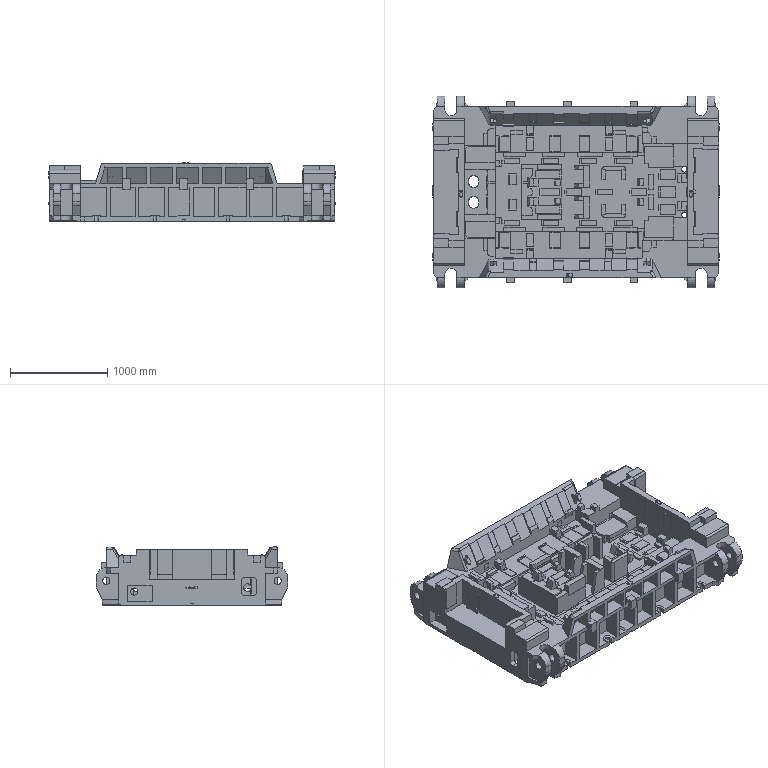Part | NX | features MAIN_BODY 2 | 1 solid | 1992 faces | box 2940 x 1970 x 600 mm | volume 853542905 mm3 | plane 1720 | cylinder 240 | spline 28 | sphere 4 | commonest cylinder face diameters 60 x93 40 x36 80 x22 50 x17 210 x16 32 x8